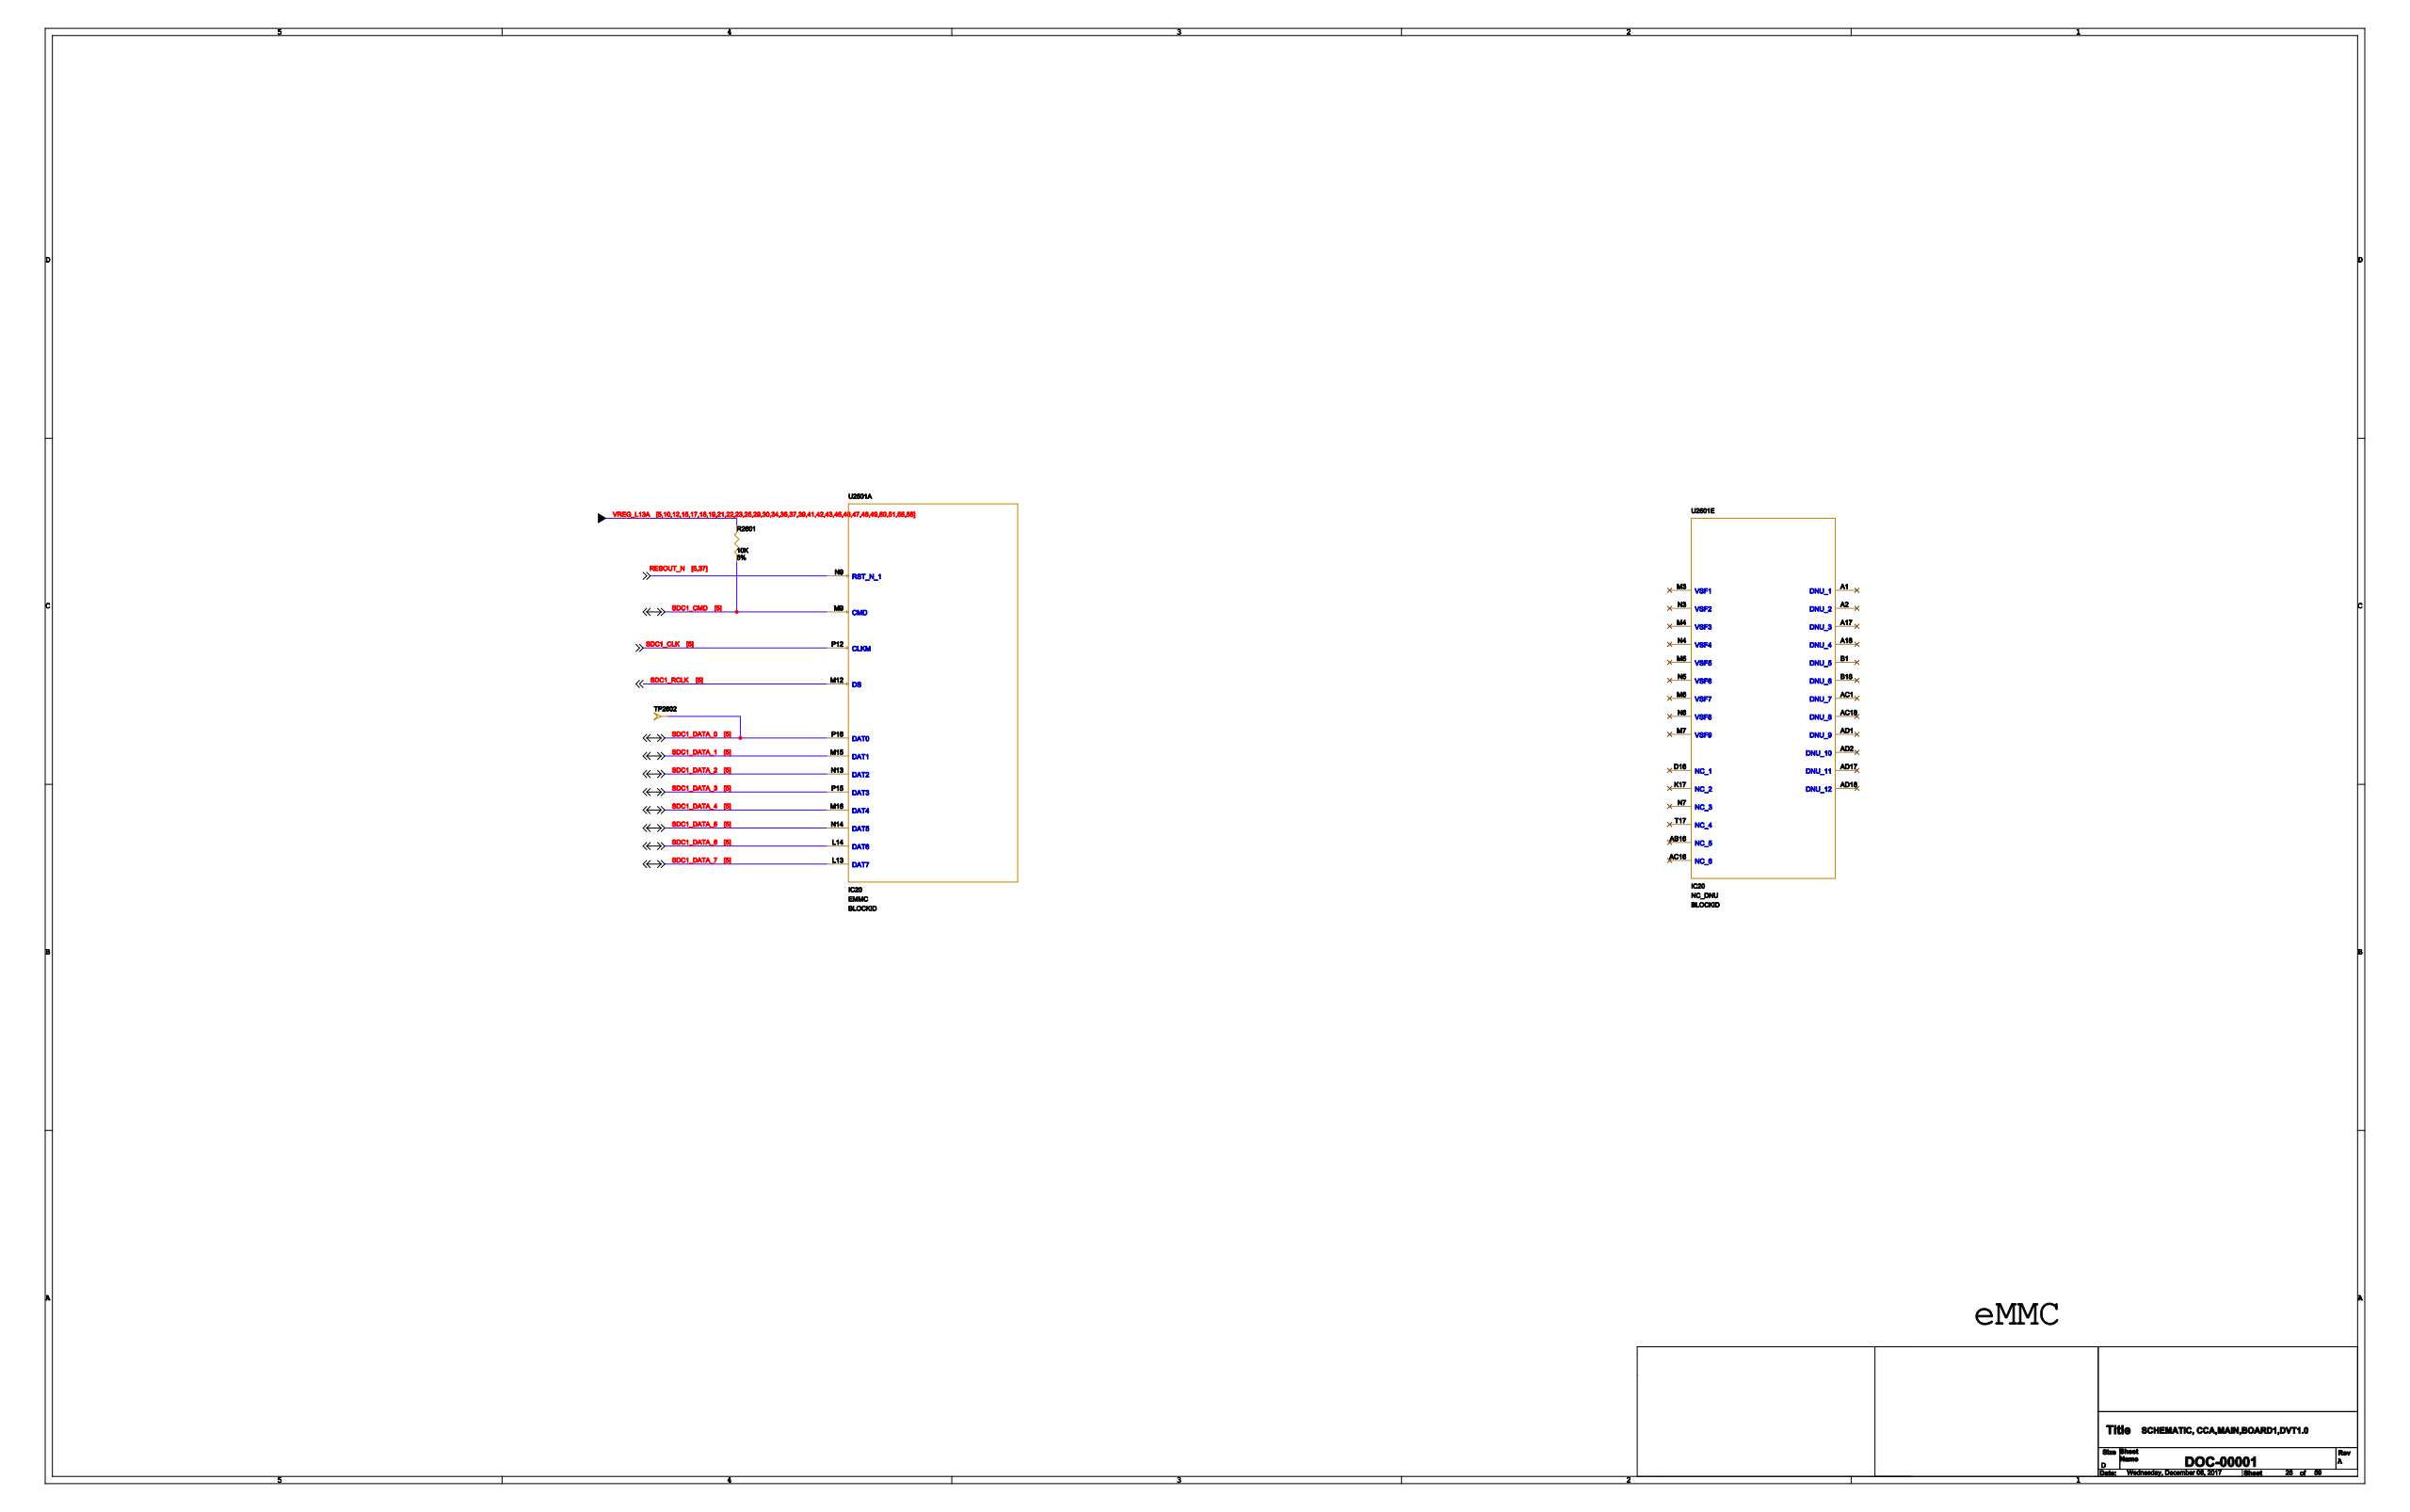Circuit board | KiCad | 1657 parts | 1365 nets | one sheet of the schematic
Parts on this sheet (reference | value | footprint):
R2601
TP2602
U2501
Nets of these parts (net: part-pin ...):
RESOUT_N: U2501-N9
VREG_L13A: R2601-1
SDC1_CMD: R2601-2 U2501-M9
SDC1_CLK: U2501-P12
SDC1_DATA_0: TP2602-1 U2501-P16
SDC1_DATA_7: U2501-L13
SDC1_DATA_6: U2501-L14
SDC1_RCLK: U2501-M12
SDC1_DATA_1: U2501-M15
SDC1_DATA_4: U2501-M16
SDC1_DATA_2: U2501-N13
SDC1_DATA_5: U2501-N14
SDC1_DATA_3: U2501-P15